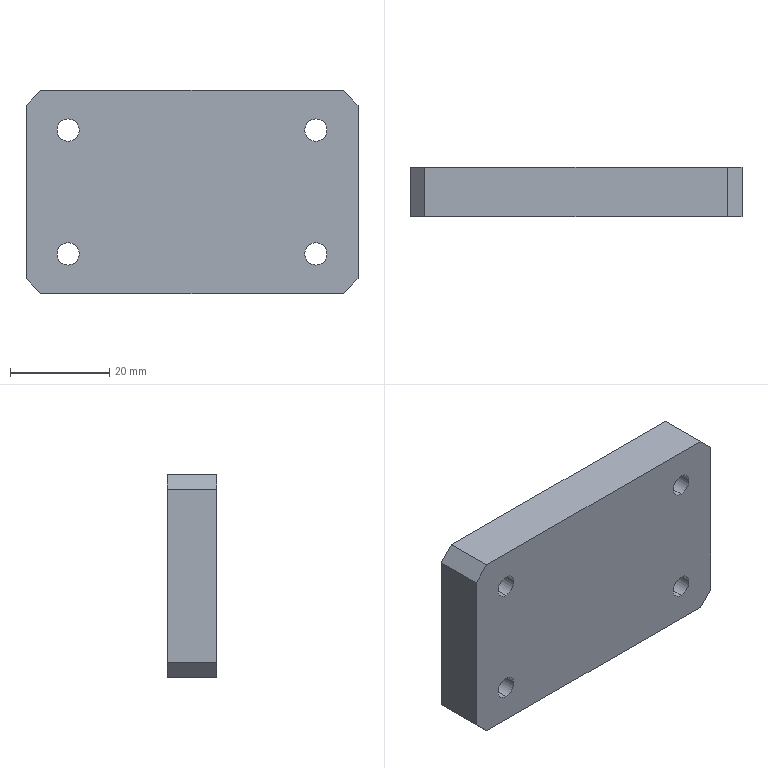Part | STEP file | 0-19 Cylinder floating plate | 1 solid | 30 faces | box 67 x 10 x 41 mm | volume 26049 mm3 | cylinder 16 | plane 14 | commonest cylinder face diameters 4.5 x8 8 x8